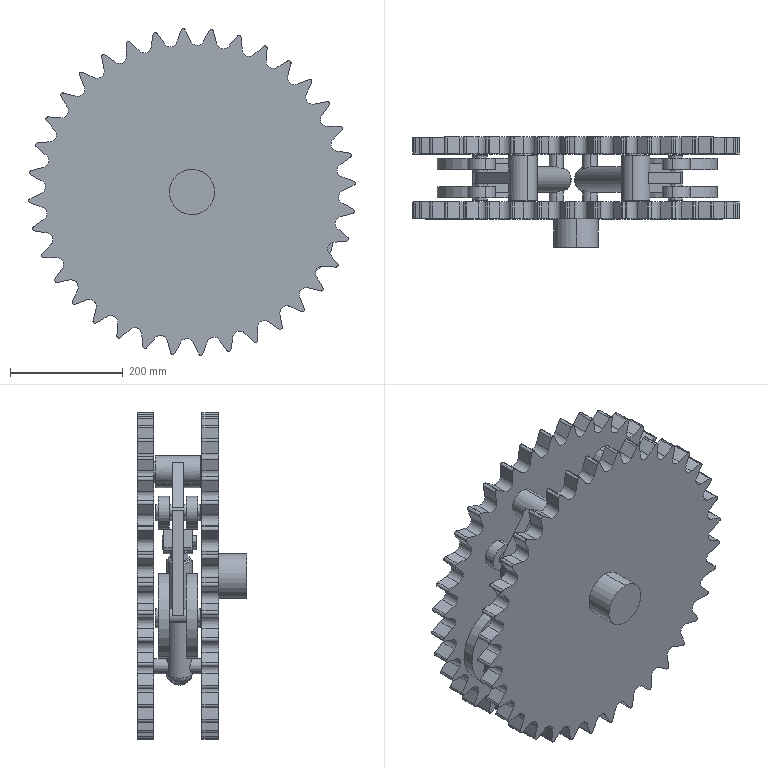Part | SolidWorks | features CompositeCurve 2, RefAxis 1 | 8 solids | 549 faces | box 579.141 x 195 x 579.141 mm | volume 17437736 mm3 | cylinder 300 | plane 237 | cone 8 | torus 4 | commonest cylinder face diameters 25 x118 8 x100 18 x16 20 x16 30 x16 50 x12